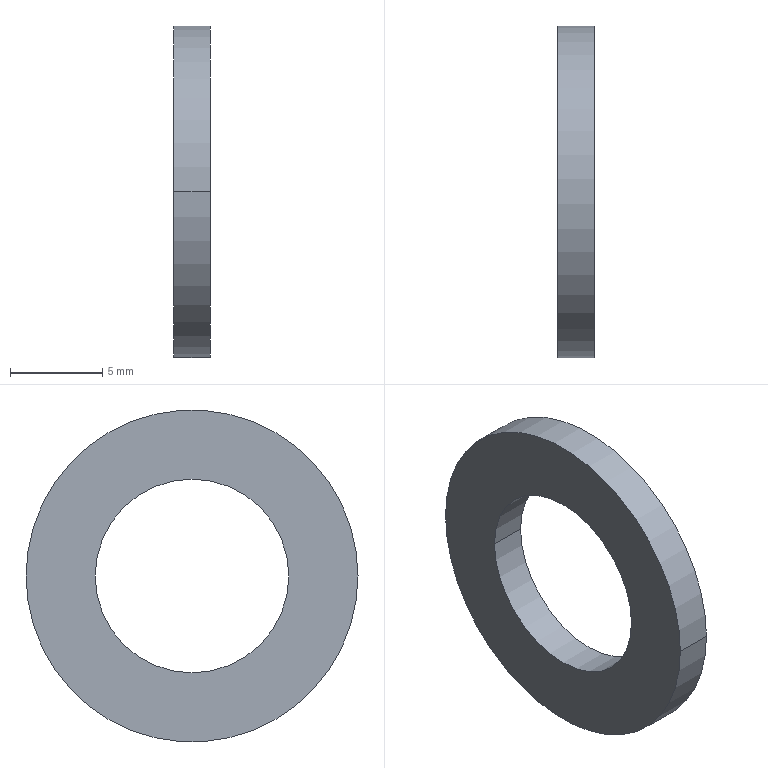Part | STEP file | KS B 1326 - 10x18 | 1 solid | 6 faces | box 2 x 18 x 18 mm | volume 335.758 mm3 | cylinder 4 | plane 2 | commonest cylinder face diameters 10.5 x2 18 x2
STEP:
#1=CARTESIAN_POINT('',(0.,0.,0.));
#2=DIRECTION('',(0.,0.,1.));
#3=DIRECTION('',(1.,0.,0.));
#4=AXIS2_PLACEMENT_3D('',#1,#2,#3);
#5=CARTESIAN_POINT('',(0.,-5.25,0.));
#6=VERTEX_POINT('',#5);
#7=CARTESIAN_POINT('',(2.,-5.25,0.));
#8=VERTEX_POINT('',#7);
#9=CARTESIAN_POINT('',(0.,-5.25,0.));
#10=DIRECTION('',(1.,0.,0.));
#11=VECTOR('',#10,1.);
#12=LINE('',#9,#11);
#13=CARTESIAN_POINT('',(0.,0.,0.));
#14=DIRECTION('',(1.,0.,0.));
#15=DIRECTION('',(0.,-1.,0.));
#16=AXIS2_PLACEMENT_3D('',#13,#14,#15);
#17=CYLINDRICAL_SURFACE('',#16,5.25);
#18=CARTESIAN_POINT('',(6.283,0.));
#19=DIRECTION('',(0.,1.));
#20=VECTOR('',#19,1.);
#21=LINE('',#18,#20);
#22=(GEOMETRIC_REPRESENTATION_CONTEXT(2)PARAMETRIC_REPRESENTATION_CONTEXT()REPRESENTATION_CONTEXT('',''));
#23=DEFINITIONAL_REPRESENTATION('',(#21),#22);
#24=PCURVE('',#17,#23);
#25=CARTESIAN_POINT('',(0.,0.,0.));
#26=DIRECTION('',(1.,0.,0.));
#27=DIRECTION('',(0.,-1.,0.));
#28=AXIS2_PLACEMENT_3D('',#25,#26,#27);
#29=CYLINDRICAL_SURFACE('',#28,5.25);
#30=CARTESIAN_POINT('',(0.,0.));
#31=DIRECTION('',(0.,1.));
#32=VECTOR('',#31,1.);
#33=LINE('',#30,#32);
#34=(GEOMETRIC_REPRESENTATION_CONTEXT(2)PARAMETRIC_REPRESENTATION_CONTEXT()REPRESENTATION_CONTEXT('',''));
#35=DEFINITIONAL_REPRESENTATION('',(#33),#34);
#36=PCURVE('',#29,#35);
#37=SURFACE_CURVE('',#12,(#24,#36),.PCURVE_S1.);
#38=EDGE_CURVE('',#6,#8,#37,.T.);
#39=ORIENTED_EDGE('',*,*,#38,.T.);
#40=CARTESIAN_POINT('',(2.,5.25,0.));
#41=VERTEX_POINT('',#40);
#42=CARTESIAN_POINT('',(2.,0.,0.));
#43=DIRECTION('',(-1.,0.,0.));
#44=DIRECTION('',(0.,-1.,0.));
#45=AXIS2_PLACEMENT_3D('',#42,#43,#44);
#46=CIRCLE('',#45,5.25);
#47=CARTESIAN_POINT('',(6.283,2.));
#48=DIRECTION('',(-1.,0.));
#49=VECTOR('',#48,1.);
#50=LINE('',#47,#49);
#51=(GEOMETRIC_REPRESENTATION_CONTEXT(2)PARAMETRIC_REPRESENTATION_CONTEXT()REPRESENTATION_CONTEXT('',''));
#52=DEFINITIONAL_REPRESENTATION('',(#50),#51);
#53=PCURVE('',#17,#52);
#54=CARTESIAN_POINT('',(2.,0.,0.));
#55=DIRECTION('',(-1.,0.,0.));
#56=DIRECTION('',(0.,0.,1.));
#57=AXIS2_PLACEMENT_3D('',#54,#55,#56);
#58=PLANE('',#57);
#59=CARTESIAN_POINT('',(0.,0.));
#60=DIRECTION('',(0.,-1.));
#61=AXIS2_PLACEMENT_2D('',#59,#60);
#62=CIRCLE('',#61,5.25);
#63=(GEOMETRIC_REPRESENTATION_CONTEXT(2)PARAMETRIC_REPRESENTATION_CONTEXT()REPRESENTATION_CONTEXT('',''));
#64=DEFINITIONAL_REPRESENTATION('',(#62),#63);
#65=PCURVE('',#58,#64);
#66=SURFACE_CURVE('',#46,(#53,#65),.PCURVE_S1.);
#67=EDGE_CURVE('',#8,#41,#66,.T.);
#68=ORIENTED_EDGE('',*,*,#67,.T.);
#69=CARTESIAN_POINT('',(0.,5.25,0.));
#70=VERTEX_POINT('',#69);
#71=CARTESIAN_POINT('',(0.,5.25,0.));
#72=DIRECTION('',(1.,0.,0.));
#73=VECTOR('',#72,1.);
#74=LINE('',#71,#73);
#75=CARTESIAN_POINT('',(3.142,0.));
#76=DIRECTION('',(0.,1.));
#77=VECTOR('',#76,1.);
#78=LINE('',#75,#77);
#79=(GEOMETRIC_REPRESENTATION_CONTEXT(2)PARAMETRIC_REPRESENTATION_CONTEXT()REPRESENTATION_CONTEXT('',''));
#80=DEFINITIONAL_REPRESENTATION('',(#78),#79);
#81=PCURVE('',#17,#80);
#82=CARTESIAN_POINT('',(3.142,0.));
#83=DIRECTION('',(0.,1.));
#84=VECTOR('',#83,1.);
#85=LINE('',#82,#84);
#86=(GEOMETRIC_REPRESENTATION_CONTEXT(2)PARAMETRIC_REPRESENTATION_CONTEXT()REPRESENTATION_CONTEXT('',''));
#87=DEFINITIONAL_REPRESENTATION('',(#85),#86);
#88=PCURVE('',#29,#87);
#89=SURFACE_CURVE('',#74,(#81,#88),.PCURVE_S1.);
#90=EDGE_CURVE('',#70,#41,#89,.T.);
#91=ORIENTED_EDGE('',*,*,#90,.F.);
#92=CARTESIAN_POINT('',(0.,0.,0.));
#93=DIRECTION('',(1.,0.,0.));
#94=DIRECTION('',(0.,-1.,0.));
#95=AXIS2_PLACEMENT_3D('',#92,#93,#94);
#96=CIRCLE('',#95,5.25);
#97=CARTESIAN_POINT('',(0.,0.));
#98=DIRECTION('',(1.,0.));
#99=VECTOR('',#98,1.);
#100=LINE('',#97,#99);
#101=(GEOMETRIC_REPRESENTATION_CONTEXT(2)PARAMETRIC_REPRESENTATION_CONTEXT()REPRESENTATION_CONTEXT('',''));
#102=DEFINITIONAL_REPRESENTATION('',(#100),#101);
#103=PCURVE('',#17,#102);
#104=CARTESIAN_POINT('',(0.,0.,0.));
#105=DIRECTION('',(-1.,0.,0.));
#106=DIRECTION('',(0.,0.,1.));
#107=AXIS2_PLACEMENT_3D('',#104,#105,#106);
#108=PLANE('',#107);
#109=CARTESIAN_POINT('',(0.,-5.25));
#110=CARTESIAN_POINT('',(-9.093,-5.25));
#111=CARTESIAN_POINT('',(-4.547,2.625));
#112=CARTESIAN_POINT('',(0.,10.5));
#113=CARTESIAN_POINT('',(4.547,2.625));
#114=CARTESIAN_POINT('',(9.093,-5.25));
#115=CARTESIAN_POINT('',(0.,-5.25));
#116=(BOUNDED_CURVE()B_SPLINE_CURVE(2,(#109,#110,#111,#112,#113,#114,#115),.UNSPECIFIED.,.T.,.F.)B_SPLINE_CURVE_WITH_KNOTS((1,2,2,2,2,1),(-2.094,0.,2.094,4.189,6.283,8.378),.UNSPECIFIED.)CURVE()GEOMETRIC_REPRESENTATION_ITEM()RATIONAL_B_SPLINE_CURVE((1.,0.5,1.,0.5,1.,0.5,1.))REPRESENTATION_ITEM(''));
#117=(GEOMETRIC_REPRESENTATION_CONTEXT(2)PARAMETRIC_REPRESENTATION_CONTEXT()REPRESENTATION_CONTEXT('',''));
#118=DEFINITIONAL_REPRESENTATION('',(#116),#117);
#119=PCURVE('',#108,#118);
#120=SURFACE_CURVE('',#96,(#103,#119),.PCURVE_S1.);
#121=EDGE_CURVE('',#70,#6,#120,.T.);
#122=ORIENTED_EDGE('',*,*,#121,.T.);
#123=EDGE_LOOP('',(#39,#68,#91,#122));
#124=FACE_BOUND('',#123,.F.);
#125=ADVANCED_FACE('',(#124),#17,.F.);
#126=CARTESIAN_POINT('',(0.,9.,0.));
#127=VERTEX_POINT('',#126);
#128=CARTESIAN_POINT('',(0.,-9.,0.));
#129=VERTEX_POINT('',#128);
#130=CARTESIAN_POINT('',(0.,0.,0.));
#131=DIRECTION('',(-1.,0.,0.));
#132=DIRECTION('',(0.,-1.,0.));
#133=AXIS2_PLACEMENT_3D('',#130,#131,#132);
#134=CIRCLE('',#133,9.);
#135=CARTESIAN_POINT('',(0.,0.,0.));
#136=DIRECTION('',(1.,0.,0.));
#137=DIRECTION('',(0.,-1.,0.));
#138=AXIS2_PLACEMENT_3D('',#135,#136,#137);
#139=CYLINDRICAL_SURFACE('',#138,9.);
#140=CARTESIAN_POINT('',(6.283,0.));
#141=DIRECTION('',(-1.,0.));
#142=VECTOR('',#141,1.);
#143=LINE('',#140,#142);
#144=(GEOMETRIC_REPRESENTATION_CONTEXT(2)PARAMETRIC_REPRESENTATION_CONTEXT()REPRESENTATION_CONTEXT('',''));
#145=DEFINITIONAL_REPRESENTATION('',(#143),#144);
#146=PCURVE('',#139,#145);
#147=CARTESIAN_POINT('',(0.,0.));
#148=DIRECTION('',(0.,-1.));
#149=AXIS2_PLACEMENT_2D('',#147,#148);
#150=CIRCLE('',#149,9.);
#151=(GEOMETRIC_REPRESENTATION_CONTEXT(2)PARAMETRIC_REPRESENTATION_CONTEXT()REPRESENTATION_CONTEXT('',''));
#152=DEFINITIONAL_REPRESENTATION('',(#150),#151);
#153=PCURVE('',#108,#152);
#154=SURFACE_CURVE('',#134,(#146,#153),.PCURVE_S1.);
#155=EDGE_CURVE('',#127,#129,#154,.T.);
#156=ORIENTED_EDGE('',*,*,#155,.F.);
#157=CARTESIAN_POINT('',(2.,9.,0.));
#158=VERTEX_POINT('',#157);
#159=CARTESIAN_POINT('',(0.,9.,0.));
#160=DIRECTION('',(1.,0.,0.));
#161=VECTOR('',#160,1.);
#162=LINE('',#159,#161);
#163=CARTESIAN_POINT('',(3.142,0.));
#164=DIRECTION('',(0.,1.));
#165=VECTOR('',#164,1.);
#166=LINE('',#163,#165);
#167=(GEOMETRIC_REPRESENTATION_CONTEXT(2)PARAMETRIC_REPRESENTATION_CONTEXT()REPRESENTATION_CONTEXT('',''));
#168=DEFINITIONAL_REPRESENTATION('',(#166),#167);
#169=PCURVE('',#139,#168);
#170=CARTESIAN_POINT('',(0.,0.,0.));
#171=DIRECTION('',(1.,0.,0.));
#172=DIRECTION('',(0.,-1.,0.));
#173=AXIS2_PLACEMENT_3D('',#170,#171,#172);
#174=CYLINDRICAL_SURFACE('',#173,9.);
#175=CARTESIAN_POINT('',(3.142,0.));
#176=DIRECTION('',(0.,1.));
#177=VECTOR('',#176,1.);
#178=LINE('',#175,#177);
#179=(GEOMETRIC_REPRESENTATION_CONTEXT(2)PARAMETRIC_REPRESENTATION_CONTEXT()REPRESENTATION_CONTEXT('',''));
#180=DEFINITIONAL_REPRESENTATION('',(#178),#179);
#181=PCURVE('',#174,#180);
#182=SURFACE_CURVE('',#162,(#169,#181),.PCURVE_S1.);
#183=EDGE_CURVE('',#127,#158,#182,.T.);
#184=ORIENTED_EDGE('',*,*,#183,.T.);
#185=CARTESIAN_POINT('',(2.,-9.,0.));
#186=VERTEX_POINT('',#185);
#187=CARTESIAN_POINT('',(2.,0.,0.));
#188=DIRECTION('',(-1.,0.,0.));
#189=DIRECTION('',(0.,-1.,0.));
#190=AXIS2_PLACEMENT_3D('',#187,#188,#189);
#191=CIRCLE('',#190,9.);
#192=CARTESIAN_POINT('',(6.283,2.));
#193=DIRECTION('',(-1.,0.));
#194=VECTOR('',#193,1.);
#195=LINE('',#192,#194);
#196=(GEOMETRIC_REPRESENTATION_CONTEXT(2)PARAMETRIC_REPRESENTATION_CONTEXT()REPRESENTATION_CONTEXT('',''));
#197=DEFINITIONAL_REPRESENTATION('',(#195),#196);
#198=PCURVE('',#139,#197);
#199=CARTESIAN_POINT('',(0.,0.));
#200=DIRECTION('',(0.,-1.));
#201=AXIS2_PLACEMENT_2D('',#199,#200);
#202=CIRCLE('',#201,9.);
#203=(GEOMETRIC_REPRESENTATION_CONTEXT(2)PARAMETRIC_REPRESENTATION_CONTEXT()REPRESENTATION_CONTEXT('',''));
#204=DEFINITIONAL_REPRESENTATION('',(#202),#203);
#205=PCURVE('',#58,#204);
#206=SURFACE_CURVE('',#191,(#198,#205),.PCURVE_S1.);
#207=EDGE_CURVE('',#158,#186,#206,.T.);
#208=ORIENTED_EDGE('',*,*,#207,.T.);
#209=CARTESIAN_POINT('',(0.,-9.,0.));
#210=DIRECTION('',(1.,0.,0.));
#211=VECTOR('',#210,1.);
#212=LINE('',#209,#211);
#213=CARTESIAN_POINT('',(0.,0.));
#214=DIRECTION('',(0.,1.));
#215=VECTOR('',#214,1.);
#216=LINE('',#213,#215);
#217=(GEOMETRIC_REPRESENTATION_CONTEXT(2)PARAMETRIC_REPRESENTATION_CONTEXT()REPRESENTATION_CONTEXT('',''));
#218=DEFINITIONAL_REPRESENTATION('',(#216),#217);
#219=PCURVE('',#139,#218);
#220=CARTESIAN_POINT('',(6.283,0.));
#221=DIRECTION('',(0.,1.));
#222=VECTOR('',#221,1.);
#223=LINE('',#220,#222);
#224=(GEOMETRIC_REPRESENTATION_CONTEXT(2)PARAMETRIC_REPRESENTATION_CONTEXT()REPRESENTATION_CONTEXT('',''));
#225=DEFINITIONAL_REPRESENTATION('',(#223),#224);
#226=PCURVE('',#174,#225);
#227=SURFACE_CURVE('',#212,(#219,#226),.PCURVE_S1.);
#228=EDGE_CURVE('',#129,#186,#227,.T.);
#229=ORIENTED_EDGE('',*,*,#228,.F.);
#230=EDGE_LOOP('',(#156,#184,#208,#229));
#231=FACE_BOUND('',#230,.T.);
#232=ADVANCED_FACE('',(#231),#139,.T.);
#233=CARTESIAN_POINT('',(0.,0.,0.));
#234=DIRECTION('',(1.,0.,0.));
#235=DIRECTION('',(0.,-1.,0.));
#236=AXIS2_PLACEMENT_3D('',#233,#234,#235);
#237=CIRCLE('',#236,5.25);
#238=CARTESIAN_POINT('',(0.,-5.25));
#239=CARTESIAN_POINT('',(-9.093,-5.25));
#240=CARTESIAN_POINT('',(-4.547,2.625));
#241=CARTESIAN_POINT('',(0.,10.5));
#242=CARTESIAN_POINT('',(4.547,2.625));
#243=CARTESIAN_POINT('',(9.093,-5.25));
#244=CARTESIAN_POINT('',(0.,-5.25));
#245=(BOUNDED_CURVE()B_SPLINE_CURVE(2,(#238,#239,#240,#241,#242,#243,#244),.UNSPECIFIED.,.T.,.F.)B_SPLINE_CURVE_WITH_KNOTS((1,2,2,2,2,1),(-2.094,0.,2.094,4.189,6.283,8.378),.UNSPECIFIED.)CURVE()GEOMETRIC_REPRESENTATION_ITEM()RATIONAL_B_SPLINE_CURVE((1.,0.5,1.,0.5,1.,0.5,1.))REPRESENTATION_ITEM(''));
#246=(GEOMETRIC_REPRESENTATION_CONTEXT(2)PARAMETRIC_REPRESENTATION_CONTEXT()REPRESENTATION_CONTEXT('',''));
#247=DEFINITIONAL_REPRESENTATION('',(#245),#246);
#248=PCURVE('',#108,#247);
#249=CARTESIAN_POINT('',(0.,0.));
#250=DIRECTION('',(1.,0.));
#251=VECTOR('',#250,1.);
#252=LINE('',#249,#251);
#253=(GEOMETRIC_REPRESENTATION_CONTEXT(2)PARAMETRIC_REPRESENTATION_CONTEXT()REPRESENTATION_CONTEXT('',''));
#254=DEFINITIONAL_REPRESENTATION('',(#252),#253);
#255=PCURVE('',#29,#254);
#256=SURFACE_CURVE('',#237,(#248,#255),.PCURVE_S1.);
#257=EDGE_CURVE('',#6,#70,#256,.T.);
#258=ORIENTED_EDGE('',*,*,#257,.T.);
#259=ORIENTED_EDGE('',*,*,#121,.T.);
#260=EDGE_LOOP('',(#258,#259));
#261=FACE_BOUND('',#260,.T.);
#262=CARTESIAN_POINT('',(0.,0.,0.));
#263=DIRECTION('',(-1.,0.,0.));
#264=DIRECTION('',(0.,-1.,0.));
#265=AXIS2_PLACEMENT_3D('',#262,#263,#264);
#266=CIRCLE('',#265,9.);
#267=CARTESIAN_POINT('',(0.,0.));
#268=DIRECTION('',(0.,-1.));
#269=AXIS2_PLACEMENT_2D('',#267,#268);
#270=CIRCLE('',#269,9.);
#271=(GEOMETRIC_REPRESENTATION_CONTEXT(2)PARAMETRIC_REPRESENTATION_CONTEXT()REPRESENTATION_CONTEXT('',''));
#272=DEFINITIONAL_REPRESENTATION('',(#270),#271);
#273=PCURVE('',#108,#272);
#274=CARTESIAN_POINT('',(6.283,0.));
#275=DIRECTION('',(-1.,0.));
#276=VECTOR('',#275,1.);
#277=LINE('',#274,#276);
#278=(GEOMETRIC_REPRESENTATION_CONTEXT(2)PARAMETRIC_REPRESENTATION_CONTEXT()REPRESENTATION_CONTEXT('',''));
#279=DEFINITIONAL_REPRESENTATION('',(#277),#278);
#280=PCURVE('',#174,#279);
#281=SURFACE_CURVE('',#266,(#273,#280),.PCURVE_S1.);
#282=EDGE_CURVE('',#129,#127,#281,.T.);
#283=ORIENTED_EDGE('',*,*,#282,.T.);
#284=ORIENTED_EDGE('',*,*,#155,.T.);
#285=EDGE_LOOP('',(#283,#284));
#286=FACE_BOUND('',#285,.T.);
#287=ADVANCED_FACE('',(#261,#286),#108,.T.);
#288=ORIENTED_EDGE('',*,*,#67,.T.);
#289=CARTESIAN_POINT('',(2.,0.,0.));
#290=DIRECTION('',(-1.,0.,0.));
#291=DIRECTION('',(0.,-1.,0.));
#292=AXIS2_PLACEMENT_3D('',#289,#290,#291);
#293=CIRCLE('',#292,5.25);
#294=CARTESIAN_POINT('',(0.,0.));
#295=DIRECTION('',(0.,-1.));
#296=AXIS2_PLACEMENT_2D('',#294,#295);
#297=CIRCLE('',#296,5.25);
#298=(GEOMETRIC_REPRESENTATION_CONTEXT(2)PARAMETRIC_REPRESENTATION_CONTEXT()REPRESENTATION_CONTEXT('',''));
#299=DEFINITIONAL_REPRESENTATION('',(#297),#298);
#300=PCURVE('',#58,#299);
#301=CARTESIAN_POINT('',(6.283,2.));
#302=DIRECTION('',(-1.,0.));
#303=VECTOR('',#302,1.);
#304=LINE('',#301,#303);
#305=(GEOMETRIC_REPRESENTATION_CONTEXT(2)PARAMETRIC_REPRESENTATION_CONTEXT()REPRESENTATION_CONTEXT('',''));
#306=DEFINITIONAL_REPRESENTATION('',(#304),#305);
#307=PCURVE('',#29,#306);
#308=SURFACE_CURVE('',#293,(#300,#307),.PCURVE_S1.);
#309=EDGE_CURVE('',#41,#8,#308,.T.);
#310=ORIENTED_EDGE('',*,*,#309,.T.);
#311=EDGE_LOOP('',(#288,#310));
#312=FACE_BOUND('',#311,.T.);
#313=CARTESIAN_POINT('',(2.,0.,0.));
#314=DIRECTION('',(-1.,0.,0.));
#315=DIRECTION('',(0.,-1.,0.));
#316=AXIS2_PLACEMENT_3D('',#313,#314,#315);
#317=CIRCLE('',#316,9.);
#318=CARTESIAN_POINT('',(0.,0.));
#319=DIRECTION('',(0.,-1.));
#320=AXIS2_PLACEMENT_2D('',#318,#319);
#321=CIRCLE('',#320,9.);
#322=(GEOMETRIC_REPRESENTATION_CONTEXT(2)PARAMETRIC_REPRESENTATION_CONTEXT()REPRESENTATION_CONTEXT('',''));
#323=DEFINITIONAL_REPRESENTATION('',(#321),#322);
#324=PCURVE('',#58,#323);
#325=CARTESIAN_POINT('',(6.283,2.));
#326=DIRECTION('',(-1.,0.));
#327=VECTOR('',#326,1.);
#328=LINE('',#325,#327);
#329=(GEOMETRIC_REPRESENTATION_CONTEXT(2)PARAMETRIC_REPRESENTATION_CONTEXT()REPRESENTATION_CONTEXT('',''));
#330=DEFINITIONAL_REPRESENTATION('',(#328),#329);
#331=PCURVE('',#174,#330);
#332=SURFACE_CURVE('',#317,(#324,#331),.PCURVE_S1.);
#333=EDGE_CURVE('',#186,#158,#332,.T.);
#334=ORIENTED_EDGE('',*,*,#333,.F.);
#335=ORIENTED_EDGE('',*,*,#207,.F.);
#336=EDGE_LOOP('',(#334,#335));
#337=FACE_BOUND('',#336,.T.);
#338=ADVANCED_FACE('',(#312,#337),#58,.F.);
#339=ORIENTED_EDGE('',*,*,#183,.F.);
#340=ORIENTED_EDGE('',*,*,#282,.F.);
#341=ORIENTED_EDGE('',*,*,#228,.T.);
#342=ORIENTED_EDGE('',*,*,#333,.T.);
#343=EDGE_LOOP('',(#339,#340,#341,#342));
#344=FACE_BOUND('',#343,.T.);
#345=ADVANCED_FACE('',(#344),#174,.T.);
#346=ORIENTED_EDGE('',*,*,#309,.T.);
#347=ORIENTED_EDGE('',*,*,#38,.F.);
#348=ORIENTED_EDGE('',*,*,#257,.T.);
#349=ORIENTED_EDGE('',*,*,#90,.T.);
#350=EDGE_LOOP('',(#346,#347,#348,#349));
#351=FACE_BOUND('',#350,.F.);
#352=ADVANCED_FACE('',(#351),#29,.F.);
#353=CLOSED_SHELL('',(#125,#232,#287,#338,#345,#352));
#354=MANIFOLD_SOLID_BREP('',#353);
#355=(LENGTH_UNIT()NAMED_UNIT(*)SI_UNIT(.MILLI.,.METRE.));
#356=UNCERTAINTY_MEASURE_WITH_UNIT(LENGTH_MEASURE(0.0000001),#355,'','');
#357=(NAMED_UNIT(*)PLANE_ANGLE_UNIT()SI_UNIT($,.RADIAN.));
#358=(NAMED_UNIT(*)SI_UNIT($,.STERADIAN.)SOLID_ANGLE_UNIT());
#359=(GEOMETRIC_REPRESENTATION_CONTEXT(3)GLOBAL_UNCERTAINTY_ASSIGNED_CONTEXT((#356))GLOBAL_UNIT_ASSIGNED_CONTEXT((#355,#357,#358))REPRESENTATION_CONTEXT('',''));
#360=ADVANCED_BREP_SHAPE_REPRESENTATION('',(#4,#354),#359);